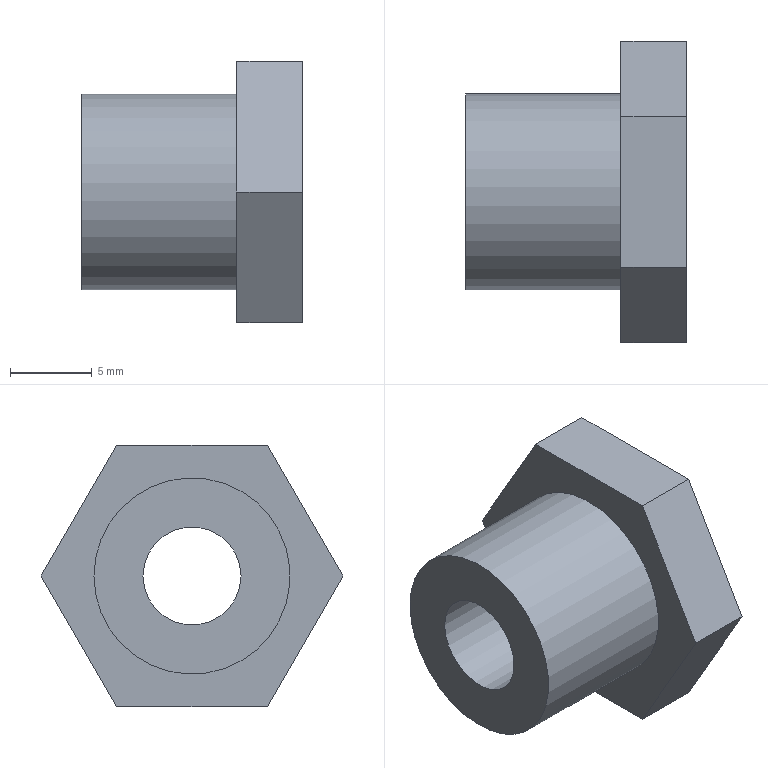Part | STEP file | 1-08.3 | 1 solid | 11 faces | box 13.5 x 18.475 x 16 mm | volume 1580 mm3 | plane 9 | cylinder 2 | commonest cylinder face diameters 6 x1 12 x1
STEP:
#1=CARTESIAN_POINT('',(0.,0.,0.));
#2=DIRECTION('',(0.,0.,1.));
#3=DIRECTION('',(1.,0.,0.));
#4=AXIS2_PLACEMENT_3D('',#1,#2,#3);
#5=CARTESIAN_POINT('',(0.,-4.619,8.));
#6=VERTEX_POINT('',#5);
#7=CARTESIAN_POINT('',(0.,4.619,8.));
#8=VERTEX_POINT('',#7);
#9=CARTESIAN_POINT('',(0.,-4.619,8.));
#10=DIRECTION('',(0.,1.,0.));
#11=VECTOR('',#10,1.);
#12=LINE('',#9,#11);
#13=CARTESIAN_POINT('',(2.,0.,8.));
#14=DIRECTION('',(0.,0.,-1.));
#15=DIRECTION('',(0.,1.,0.));
#16=AXIS2_PLACEMENT_3D('',#13,#14,#15);
#17=PLANE('',#16);
#18=CARTESIAN_POINT('',(-4.619,-2.));
#19=DIRECTION('',(1.,0.));
#20=VECTOR('',#19,1.);
#21=LINE('',#18,#20);
#22=(GEOMETRIC_REPRESENTATION_CONTEXT(2)PARAMETRIC_REPRESENTATION_CONTEXT()REPRESENTATION_CONTEXT('',''));
#23=DEFINITIONAL_REPRESENTATION('',(#21),#22);
#24=PCURVE('',#17,#23);
#25=CARTESIAN_POINT('',(0.,0.,1.238));
#26=DIRECTION('',(-1.,0.,0.));
#27=DIRECTION('',(0.,0.,1.));
#28=AXIS2_PLACEMENT_3D('',#25,#26,#27);
#29=PLANE('',#28);
#30=CARTESIAN_POINT('',(6.762,-4.619));
#31=DIRECTION('',(0.,1.));
#32=VECTOR('',#31,1.);
#33=LINE('',#30,#32);
#34=(GEOMETRIC_REPRESENTATION_CONTEXT(2)PARAMETRIC_REPRESENTATION_CONTEXT()REPRESENTATION_CONTEXT('',''));
#35=DEFINITIONAL_REPRESENTATION('',(#33),#34);
#36=PCURVE('',#29,#35);
#37=SURFACE_CURVE('',#12,(#24,#36),.PCURVE_S1.);
#38=EDGE_CURVE('',#6,#8,#37,.T.);
#39=ORIENTED_EDGE('',*,*,#38,.T.);
#40=CARTESIAN_POINT('',(4.,4.619,8.));
#41=VERTEX_POINT('',#40);
#42=CARTESIAN_POINT('',(0.,4.619,8.));
#43=DIRECTION('',(1.,0.,0.));
#44=VECTOR('',#43,1.);
#45=LINE('',#42,#44);
#46=CARTESIAN_POINT('',(4.619,-2.));
#47=DIRECTION('',(0.,1.));
#48=VECTOR('',#47,1.);
#49=LINE('',#46,#48);
#50=(GEOMETRIC_REPRESENTATION_CONTEXT(2)PARAMETRIC_REPRESENTATION_CONTEXT()REPRESENTATION_CONTEXT('',''));
#51=DEFINITIONAL_REPRESENTATION('',(#49),#50);
#52=PCURVE('',#17,#51);
#53=CARTESIAN_POINT('',(2.,6.928,4.));
#54=DIRECTION('',(0.,-0.866,-0.5));
#55=DIRECTION('',(0.,0.5,-0.866));
#56=AXIS2_PLACEMENT_3D('',#53,#54,#55);
#57=PLANE('',#56);
#58=CARTESIAN_POINT('',(-4.619,-2.));
#59=DIRECTION('',(0.,1.));
#60=VECTOR('',#59,1.);
#61=LINE('',#58,#60);
#62=(GEOMETRIC_REPRESENTATION_CONTEXT(2)PARAMETRIC_REPRESENTATION_CONTEXT()REPRESENTATION_CONTEXT('',''));
#63=DEFINITIONAL_REPRESENTATION('',(#61),#62);
#64=PCURVE('',#57,#63);
#65=SURFACE_CURVE('',#45,(#52,#64),.PCURVE_S1.);
#66=EDGE_CURVE('',#8,#41,#65,.T.);
#67=ORIENTED_EDGE('',*,*,#66,.T.);
#68=CARTESIAN_POINT('',(4.,-4.619,8.));
#69=VERTEX_POINT('',#68);
#70=CARTESIAN_POINT('',(4.,-4.619,8.));
#71=DIRECTION('',(0.,1.,0.));
#72=VECTOR('',#71,1.);
#73=LINE('',#70,#72);
#74=CARTESIAN_POINT('',(-4.619,2.));
#75=DIRECTION('',(1.,0.));
#76=VECTOR('',#75,1.);
#77=LINE('',#74,#76);
#78=(GEOMETRIC_REPRESENTATION_CONTEXT(2)PARAMETRIC_REPRESENTATION_CONTEXT()REPRESENTATION_CONTEXT('',''));
#79=DEFINITIONAL_REPRESENTATION('',(#77),#78);
#80=PCURVE('',#17,#79);
#81=CARTESIAN_POINT('',(4.,0.,1.238));
#82=DIRECTION('',(-1.,0.,0.));
#83=DIRECTION('',(0.,0.,1.));
#84=AXIS2_PLACEMENT_3D('',#81,#82,#83);
#85=PLANE('',#84);
#86=CARTESIAN_POINT('',(6.762,-4.619));
#87=DIRECTION('',(0.,1.));
#88=VECTOR('',#87,1.);
#89=LINE('',#86,#88);
#90=(GEOMETRIC_REPRESENTATION_CONTEXT(2)PARAMETRIC_REPRESENTATION_CONTEXT()REPRESENTATION_CONTEXT('',''));
#91=DEFINITIONAL_REPRESENTATION('',(#89),#90);
#92=PCURVE('',#85,#91);
#93=SURFACE_CURVE('',#73,(#80,#92),.PCURVE_S1.);
#94=EDGE_CURVE('',#69,#41,#93,.T.);
#95=ORIENTED_EDGE('',*,*,#94,.F.);
#96=CARTESIAN_POINT('',(0.,-4.619,8.));
#97=DIRECTION('',(1.,0.,0.));
#98=VECTOR('',#97,1.);
#99=LINE('',#96,#98);
#100=CARTESIAN_POINT('',(-4.619,-2.));
#101=DIRECTION('',(0.,1.));
#102=VECTOR('',#101,1.);
#103=LINE('',#100,#102);
#104=(GEOMETRIC_REPRESENTATION_CONTEXT(2)PARAMETRIC_REPRESENTATION_CONTEXT()REPRESENTATION_CONTEXT('',''));
#105=DEFINITIONAL_REPRESENTATION('',(#103),#104);
#106=PCURVE('',#17,#105);
#107=CARTESIAN_POINT('',(2.,-6.928,4.));
#108=DIRECTION('',(0.,0.866,-0.5));
#109=DIRECTION('',(0.,0.5,0.866));
#110=AXIS2_PLACEMENT_3D('',#107,#108,#109);
#111=PLANE('',#110);
#112=CARTESIAN_POINT('',(4.619,-2.));
#113=DIRECTION('',(0.,1.));
#114=VECTOR('',#113,1.);
#115=LINE('',#112,#114);
#116=(GEOMETRIC_REPRESENTATION_CONTEXT(2)PARAMETRIC_REPRESENTATION_CONTEXT()REPRESENTATION_CONTEXT('',''));
#117=DEFINITIONAL_REPRESENTATION('',(#115),#116);
#118=PCURVE('',#111,#117);
#119=SURFACE_CURVE('',#99,(#106,#118),.PCURVE_S1.);
#120=EDGE_CURVE('',#6,#69,#119,.T.);
#121=ORIENTED_EDGE('',*,*,#120,.F.);
#122=EDGE_LOOP('',(#39,#67,#95,#121));
#123=FACE_BOUND('',#122,.F.);
#124=ADVANCED_FACE('',(#123),#17,.F.);
#125=CARTESIAN_POINT('',(0.,9.238,0.));
#126=VERTEX_POINT('',#125);
#127=CARTESIAN_POINT('',(0.,4.619,8.));
#128=DIRECTION('',(0.,0.5,-0.866));
#129=VECTOR('',#128,1.);
#130=LINE('',#127,#129);
#131=CARTESIAN_POINT('',(-4.619,-2.));
#132=DIRECTION('',(1.,0.));
#133=VECTOR('',#132,1.);
#134=LINE('',#131,#133);
#135=(GEOMETRIC_REPRESENTATION_CONTEXT(2)PARAMETRIC_REPRESENTATION_CONTEXT()REPRESENTATION_CONTEXT('',''));
#136=DEFINITIONAL_REPRESENTATION('',(#134),#135);
#137=PCURVE('',#57,#136);
#138=CARTESIAN_POINT('',(6.762,4.619));
#139=DIRECTION('',(-0.866,0.5));
#140=VECTOR('',#139,1.);
#141=LINE('',#138,#140);
#142=(GEOMETRIC_REPRESENTATION_CONTEXT(2)PARAMETRIC_REPRESENTATION_CONTEXT()REPRESENTATION_CONTEXT('',''));
#143=DEFINITIONAL_REPRESENTATION('',(#141),#142);
#144=PCURVE('',#29,#143);
#145=SURFACE_CURVE('',#130,(#137,#144),.PCURVE_S1.);
#146=EDGE_CURVE('',#8,#126,#145,.T.);
#147=ORIENTED_EDGE('',*,*,#146,.T.);
#148=CARTESIAN_POINT('',(4.,9.238,0.));
#149=VERTEX_POINT('',#148);
#150=CARTESIAN_POINT('',(0.,9.238,0.));
#151=DIRECTION('',(1.,0.,0.));
#152=VECTOR('',#151,1.);
#153=LINE('',#150,#152);
#154=CARTESIAN_POINT('',(4.619,-2.));
#155=DIRECTION('',(0.,1.));
#156=VECTOR('',#155,1.);
#157=LINE('',#154,#156);
#158=(GEOMETRIC_REPRESENTATION_CONTEXT(2)PARAMETRIC_REPRESENTATION_CONTEXT()REPRESENTATION_CONTEXT('',''));
#159=DEFINITIONAL_REPRESENTATION('',(#157),#158);
#160=PCURVE('',#57,#159);
#161=CARTESIAN_POINT('',(2.,6.928,-4.));
#162=DIRECTION('',(0.,-0.866,0.5));
#163=DIRECTION('',(0.,-0.5,-0.866));
#164=AXIS2_PLACEMENT_3D('',#161,#162,#163);
#165=PLANE('',#164);
#166=CARTESIAN_POINT('',(-4.619,-2.));
#167=DIRECTION('',(0.,1.));
#168=VECTOR('',#167,1.);
#169=LINE('',#166,#168);
#170=(GEOMETRIC_REPRESENTATION_CONTEXT(2)PARAMETRIC_REPRESENTATION_CONTEXT()REPRESENTATION_CONTEXT('',''));
#171=DEFINITIONAL_REPRESENTATION('',(#169),#170);
#172=PCURVE('',#165,#171);
#173=SURFACE_CURVE('',#153,(#160,#172),.PCURVE_S1.);
#174=EDGE_CURVE('',#126,#149,#173,.T.);
#175=ORIENTED_EDGE('',*,*,#174,.T.);
#176=CARTESIAN_POINT('',(4.,4.619,8.));
#177=DIRECTION('',(0.,0.5,-0.866));
#178=VECTOR('',#177,1.);
#179=LINE('',#176,#178);
#180=CARTESIAN_POINT('',(-4.619,2.));
#181=DIRECTION('',(1.,0.));
#182=VECTOR('',#181,1.);
#183=LINE('',#180,#182);
#184=(GEOMETRIC_REPRESENTATION_CONTEXT(2)PARAMETRIC_REPRESENTATION_CONTEXT()REPRESENTATION_CONTEXT('',''));
#185=DEFINITIONAL_REPRESENTATION('',(#183),#184);
#186=PCURVE('',#57,#185);
#187=CARTESIAN_POINT('',(6.762,4.619));
#188=DIRECTION('',(-0.866,0.5));
#189=VECTOR('',#188,1.);
#190=LINE('',#187,#189);
#191=(GEOMETRIC_REPRESENTATION_CONTEXT(2)PARAMETRIC_REPRESENTATION_CONTEXT()REPRESENTATION_CONTEXT('',''));
#192=DEFINITIONAL_REPRESENTATION('',(#190),#191);
#193=PCURVE('',#85,#192);
#194=SURFACE_CURVE('',#179,(#186,#193),.PCURVE_S1.);
#195=EDGE_CURVE('',#41,#149,#194,.T.);
#196=ORIENTED_EDGE('',*,*,#195,.F.);
#197=ORIENTED_EDGE('',*,*,#66,.F.);
#198=EDGE_LOOP('',(#147,#175,#196,#197));
#199=FACE_BOUND('',#198,.F.);
#200=ADVANCED_FACE('',(#199),#57,.F.);
#201=CARTESIAN_POINT('',(0.,4.619,-8.));
#202=VERTEX_POINT('',#201);
#203=CARTESIAN_POINT('',(0.,9.238,0.));
#204=DIRECTION('',(0.,-0.5,-0.866));
#205=VECTOR('',#204,1.);
#206=LINE('',#203,#205);
#207=CARTESIAN_POINT('',(-4.619,-2.));
#208=DIRECTION('',(1.,0.));
#209=VECTOR('',#208,1.);
#210=LINE('',#207,#209);
#211=(GEOMETRIC_REPRESENTATION_CONTEXT(2)PARAMETRIC_REPRESENTATION_CONTEXT()REPRESENTATION_CONTEXT('',''));
#212=DEFINITIONAL_REPRESENTATION('',(#210),#211);
#213=PCURVE('',#165,#212);
#214=CARTESIAN_POINT('',(-1.238,9.238));
#215=DIRECTION('',(-0.866,-0.5));
#216=VECTOR('',#215,1.);
#217=LINE('',#214,#216);
#218=(GEOMETRIC_REPRESENTATION_CONTEXT(2)PARAMETRIC_REPRESENTATION_CONTEXT()REPRESENTATION_CONTEXT('',''));
#219=DEFINITIONAL_REPRESENTATION('',(#217),#218);
#220=PCURVE('',#29,#219);
#221=SURFACE_CURVE('',#206,(#213,#220),.PCURVE_S1.);
#222=EDGE_CURVE('',#126,#202,#221,.T.);
#223=ORIENTED_EDGE('',*,*,#222,.T.);
#224=CARTESIAN_POINT('',(4.,4.619,-8.));
#225=VERTEX_POINT('',#224);
#226=CARTESIAN_POINT('',(0.,4.619,-8.));
#227=DIRECTION('',(1.,0.,0.));
#228=VECTOR('',#227,1.);
#229=LINE('',#226,#228);
#230=CARTESIAN_POINT('',(4.619,-2.));
#231=DIRECTION('',(0.,1.));
#232=VECTOR('',#231,1.);
#233=LINE('',#230,#232);
#234=(GEOMETRIC_REPRESENTATION_CONTEXT(2)PARAMETRIC_REPRESENTATION_CONTEXT()REPRESENTATION_CONTEXT('',''));
#235=DEFINITIONAL_REPRESENTATION('',(#233),#234);
#236=PCURVE('',#165,#235);
#237=CARTESIAN_POINT('',(2.,0.,-8.));
#238=DIRECTION('',(0.,0.,1.));
#239=DIRECTION('',(0.,-1.,0.));
#240=AXIS2_PLACEMENT_3D('',#237,#238,#239);
#241=PLANE('',#240);
#242=CARTESIAN_POINT('',(-4.619,-2.));
#243=DIRECTION('',(0.,1.));
#244=VECTOR('',#243,1.);
#245=LINE('',#242,#244);
#246=(GEOMETRIC_REPRESENTATION_CONTEXT(2)PARAMETRIC_REPRESENTATION_CONTEXT()REPRESENTATION_CONTEXT('',''));
#247=DEFINITIONAL_REPRESENTATION('',(#245),#246);
#248=PCURVE('',#241,#247);
#249=SURFACE_CURVE('',#229,(#236,#248),.PCURVE_S1.);
#250=EDGE_CURVE('',#202,#225,#249,.T.);
#251=ORIENTED_EDGE('',*,*,#250,.T.);
#252=CARTESIAN_POINT('',(4.,9.238,0.));
#253=DIRECTION('',(0.,-0.5,-0.866));
#254=VECTOR('',#253,1.);
#255=LINE('',#252,#254);
#256=CARTESIAN_POINT('',(-4.619,2.));
#257=DIRECTION('',(1.,0.));
#258=VECTOR('',#257,1.);
#259=LINE('',#256,#258);
#260=(GEOMETRIC_REPRESENTATION_CONTEXT(2)PARAMETRIC_REPRESENTATION_CONTEXT()REPRESENTATION_CONTEXT('',''));
#261=DEFINITIONAL_REPRESENTATION('',(#259),#260);
#262=PCURVE('',#165,#261);
#263=CARTESIAN_POINT('',(-1.238,9.238));
#264=DIRECTION('',(-0.866,-0.5));
#265=VECTOR('',#264,1.);
#266=LINE('',#263,#265);
#267=(GEOMETRIC_REPRESENTATION_CONTEXT(2)PARAMETRIC_REPRESENTATION_CONTEXT()REPRESENTATION_CONTEXT('',''));
#268=DEFINITIONAL_REPRESENTATION('',(#266),#267);
#269=PCURVE('',#85,#268);
#270=SURFACE_CURVE('',#255,(#262,#269),.PCURVE_S1.);
#271=EDGE_CURVE('',#149,#225,#270,.T.);
#272=ORIENTED_EDGE('',*,*,#271,.F.);
#273=ORIENTED_EDGE('',*,*,#174,.F.);
#274=EDGE_LOOP('',(#223,#251,#272,#273));
#275=FACE_BOUND('',#274,.F.);
#276=ADVANCED_FACE('',(#275),#165,.F.);
#277=CARTESIAN_POINT('',(0.,-4.619,-8.));
#278=VERTEX_POINT('',#277);
#279=CARTESIAN_POINT('',(0.,4.619,-8.));
#280=DIRECTION('',(0.,-1.,0.));
#281=VECTOR('',#280,1.);
#282=LINE('',#279,#281);
#283=CARTESIAN_POINT('',(-4.619,-2.));
#284=DIRECTION('',(1.,0.));
#285=VECTOR('',#284,1.);
#286=LINE('',#283,#285);
#287=(GEOMETRIC_REPRESENTATION_CONTEXT(2)PARAMETRIC_REPRESENTATION_CONTEXT()REPRESENTATION_CONTEXT('',''));
#288=DEFINITIONAL_REPRESENTATION('',(#286),#287);
#289=PCURVE('',#241,#288);
#290=CARTESIAN_POINT('',(-9.238,4.619));
#291=DIRECTION('',(0.,-1.));
#292=VECTOR('',#291,1.);
#293=LINE('',#290,#292);
#294=(GEOMETRIC_REPRESENTATION_CONTEXT(2)PARAMETRIC_REPRESENTATION_CONTEXT()REPRESENTATION_CONTEXT('',''));
#295=DEFINITIONAL_REPRESENTATION('',(#293),#294);
#296=PCURVE('',#29,#295);
#297=SURFACE_CURVE('',#282,(#289,#296),.PCURVE_S1.);
#298=EDGE_CURVE('',#202,#278,#297,.T.);
#299=ORIENTED_EDGE('',*,*,#298,.T.);
#300=CARTESIAN_POINT('',(4.,-4.619,-8.));
#301=VERTEX_POINT('',#300);
#302=CARTESIAN_POINT('',(0.,-4.619,-8.));
#303=DIRECTION('',(1.,0.,0.));
#304=VECTOR('',#303,1.);
#305=LINE('',#302,#304);
#306=CARTESIAN_POINT('',(4.619,-2.));
#307=DIRECTION('',(0.,1.));
#308=VECTOR('',#307,1.);
#309=LINE('',#306,#308);
#310=(GEOMETRIC_REPRESENTATION_CONTEXT(2)PARAMETRIC_REPRESENTATION_CONTEXT()REPRESENTATION_CONTEXT('',''));
#311=DEFINITIONAL_REPRESENTATION('',(#309),#310);
#312=PCURVE('',#241,#311);
#313=CARTESIAN_POINT('',(2.,-6.928,-4.));
#314=DIRECTION('',(0.,0.866,0.5));
#315=DIRECTION('',(0.,-0.5,0.866));
#316=AXIS2_PLACEMENT_3D('',#313,#314,#315);
#317=PLANE('',#316);
#318=CARTESIAN_POINT('',(-4.619,-2.));
#319=DIRECTION('',(0.,1.));
#320=VECTOR('',#319,1.);
#321=LINE('',#318,#320);
#322=(GEOMETRIC_REPRESENTATION_CONTEXT(2)PARAMETRIC_REPRESENTATION_CONTEXT()REPRESENTATION_CONTEXT('',''));
#323=DEFINITIONAL_REPRESENTATION('',(#321),#322);
#324=PCURVE('',#317,#323);
#325=SURFACE_CURVE('',#305,(#312,#324),.PCURVE_S1.);
#326=EDGE_CURVE('',#278,#301,#325,.T.);
#327=ORIENTED_EDGE('',*,*,#326,.T.);
#328=CARTESIAN_POINT('',(4.,4.619,-8.));
#329=DIRECTION('',(0.,-1.,0.));
#330=VECTOR('',#329,1.);
#331=LINE('',#328,#330);
#332=CARTESIAN_POINT('',(-4.619,2.));
#333=DIRECTION('',(1.,0.));
#334=VECTOR('',#333,1.);
#335=LINE('',#332,#334);
#336=(GEOMETRIC_REPRESENTATION_CONTEXT(2)PARAMETRIC_REPRESENTATION_CONTEXT()REPRESENTATION_CONTEXT('',''));
#337=DEFINITIONAL_REPRESENTATION('',(#335),#336);
#338=PCURVE('',#241,#337);
#339=CARTESIAN_POINT('',(-9.238,4.619));
#340=DIRECTION('',(0.,-1.));
#341=VECTOR('',#340,1.);
#342=LINE('',#339,#341);
#343=(GEOMETRIC_REPRESENTATION_CONTEXT(2)PARAMETRIC_REPRESENTATION_CONTEXT()REPRESENTATION_CONTEXT('',''));
#344=DEFINITIONAL_REPRESENTATION('',(#342),#343);
#345=PCURVE('',#85,#344);
#346=SURFACE_CURVE('',#331,(#338,#345),.PCURVE_S1.);
#347=EDGE_CURVE('',#225,#301,#346,.T.);
#348=ORIENTED_EDGE('',*,*,#347,.F.);
#349=ORIENTED_EDGE('',*,*,#250,.F.);
#350=EDGE_LOOP('',(#299,#327,#348,#349));
#351=FACE_BOUND('',#350,.F.);
#352=ADVANCED_FACE('',(#351),#241,.F.);
#353=CARTESIAN_POINT('',(0.,-9.238,0.));
#354=VERTEX_POINT('',#353);
#355=CARTESIAN_POINT('',(0.,-4.619,-8.));
#356=DIRECTION('',(0.,-0.5,0.866));
#357=VECTOR('',#356,1.);
#358=LINE('',#355,#357);
#359=CARTESIAN_POINT('',(-4.619,-2.));
#360=DIRECTION('',(1.,0.));
#361=VECTOR('',#360,1.);
#362=LINE('',#359,#361);
#363=(GEOMETRIC_REPRESENTATION_CONTEXT(2)PARAMETRIC_REPRESENTATION_CONTEXT()REPRESENTATION_CONTEXT('',''));
#364=DEFINITIONAL_REPRESENTATION('',(#362),#363);
#365=PCURVE('',#317,#364);
#366=CARTESIAN_POINT('',(-9.238,-4.619));
#367=DIRECTION('',(0.866,-0.5));
#368=VECTOR('',#367,1.);
#369=LINE('',#366,#368);
#370=(GEOMETRIC_REPRESENTATION_CONTEXT(2)PARAMETRIC_REPRESENTATION_CONTEXT()REPRESENTATION_CONTEXT('',''));
#371=DEFINITIONAL_REPRESENTATION('',(#369),#370);
#372=PCURVE('',#29,#371);
#373=SURFACE_CURVE('',#358,(#365,#372),.PCURVE_S1.);
#374=EDGE_CURVE('',#278,#354,#373,.T.);
#375=ORIENTED_EDGE('',*,*,#374,.T.);
#376=CARTESIAN_POINT('',(4.,-9.238,0.));
#377=VERTEX_POINT('',#376);
#378=CARTESIAN_POINT('',(0.,-9.238,0.));
#379=DIRECTION('',(1.,0.,0.));
#380=VECTOR('',#379,1.);
#381=LINE('',#378,#380);
#382=CARTESIAN_POINT('',(4.619,-2.));
#383=DIRECTION('',(0.,1.));
#384=VECTOR('',#383,1.);
#385=LINE('',#382,#384);
#386=(GEOMETRIC_REPRESENTATION_CONTEXT(2)PARAMETRIC_REPRESENTATION_CONTEXT()REPRESENTATION_CONTEXT('',''));
#387=DEFINITIONAL_REPRESENTATION('',(#385),#386);
#388=PCURVE('',#317,#387);
#389=CARTESIAN_POINT('',(-4.619,-2.));
#390=DIRECTION('',(0.,1.));
#391=VECTOR('',#390,1.);
#392=LINE('',#389,#391);
#393=(GEOMETRIC_REPRESENTATION_CONTEXT(2)PARAMETRIC_REPRESENTATION_CONTEXT()REPRESENTATION_CONTEXT('',''));
#394=DEFINITIONAL_REPRESENTATION('',(#392),#393);
#395=PCURVE('',#111,#394);
#396=SURFACE_CURVE('',#381,(#388,#395),.PCURVE_S1.);
#397=EDGE_CURVE('',#354,#377,#396,.T.);
#398=ORIENTED_EDGE('',*,*,#397,.T.);
#399=CARTESIAN_POINT('',(4.,-4.619,-8.));
#400=DIRECTION('',(0.,-0.5,0.866));
#401=VECTOR('',#400,1.);
#402=LINE('',#399,#401);
#403=CARTESIAN_POINT('',(-4.619,2.));
#404=DIRECTION('',(1.,0.));
#405=VECTOR('',#404,1.);
#406=LINE('',#403,#405);
#407=(GEOMETRIC_REPRESENTATION_CONTEXT(2)PARAMETRIC_REPRESENTATION_CONTEXT()REPRESENTATION_CONTEXT('',''));
#408=DEFINITIONAL_REPRESENTATION('',(#406),#407);
#409=PCURVE('',#317,#408);
#410=CARTESIAN_POINT('',(-9.238,-4.619));
#411=DIRECTION('',(0.866,-0.5));
#412=VECTOR('',#411,1.);
#413=LINE('',#410,#412);
#414=(GEOMETRIC_REPRESENTATION_CONTEXT(2)PARAMETRIC_REPRESENTATION_CONTEXT()REPRESENTATION_CONTEXT('',''));
#415=DEFINITIONAL_REPRESENTATION('',(#413),#414);
#416=PCURVE('',#85,#415);
#417=SURFACE_CURVE('',#402,(#409,#416),.PCURVE_S1.);
#418=EDGE_CURVE('',#301,#377,#417,.T.);
#419=ORIENTED_EDGE('',*,*,#418,.F.);
#420=ORIENTED_EDGE('',*,*,#326,.F.);
#421=EDGE_LOOP('',(#375,#398,#419,#420));
#422=FACE_BOUND('',#421,.F.);
#423=ADVANCED_FACE('',(#422),#317,.F.);
#424=CARTESIAN_POINT('',(0.,-9.238,0.));
#425=DIRECTION('',(0.,0.5,0.866));
#426=VECTOR('',#425,1.);
#427=LINE('',#424,#426);
#428=CARTESIAN_POINT('',(-4.619,-2.));
#429=DIRECTION('',(1.,0.));
#430=VECTOR('',#429,1.);
#431=LINE('',#428,#430);
#432=(GEOMETRIC_REPRESENTATION_CONTEXT(2)PARAMETRIC_REPRESENTATION_CONTEXT()REPRESENTATION_CONTEXT('',''));
#433=DEFINITIONAL_REPRESENTATION('',(#431),#432);
#434=PCURVE('',#111,#433);
#435=CARTESIAN_POINT('',(-1.238,-9.238));
#436=DIRECTION('',(0.866,0.5));
#437=VECTOR('',#436,1.);
#438=LINE('',#435,#437);
#439=(GEOMETRIC_REPRESENTATION_CONTEXT(2)PARAMETRIC_REPRESENTATION_CONTEXT()REPRESENTATION_CONTEXT('',''));
#440=DEFINITIONAL_REPRESENTATION('',(#438),#439);
#441=PCURVE('',#29,#440);
#442=SURFACE_CURVE('',#427,(#434,#441),.PCURVE_S1.);
#443=EDGE_CURVE('',#354,#6,#442,.T.);
#444=ORIENTED_EDGE('',*,*,#443,.T.);
#445=ORIENTED_EDGE('',*,*,#120,.T.);
#446=CARTESIAN_POINT('',(4.,-9.238,0.));
#447=DIRECTION('',(0.,0.5,0.866));
#448=VECTOR('',#447,1.);
#449=LINE('',#446,#448);
#450=CARTESIAN_POINT('',(-4.619,2.));
#451=DIRECTION('',(1.,0.));
#452=VECTOR('',#451,1.);
#453=LINE('',#450,#452);
#454=(GEOMETRIC_REPRESENTATION_CONTEXT(2)PARAMETRIC_REPRESENTATION_CONTEXT()REPRESENTATION_CONTEXT('',''));
#455=DEFINITIONAL_REPRESENTATION('',(#453),#454);
#456=PCURVE('',#111,#455);
#457=CARTESIAN_POINT('',(-1.238,-9.238));
#458=DIRECTION('',(0.866,0.5));
#459=VECTOR('',#458,1.);
#460=LINE('',#457,#459);
#461=(GEOMETRIC_REPRESENTATION_CONTEXT(2)PARAMETRIC_REPRESENTATION_CONTEXT()REPRESENTATION_CONTEXT('',''));
#462=DEFINITIONAL_REPRESENTATION('',(#460),#461);
#463=PCURVE('',#85,#462);
#464=SURFACE_CURVE('',#449,(#456,#463),.PCURVE_S1.);
#465=EDGE_CURVE('',#377,#69,#464,.T.);
#466=ORIENTED_EDGE('',*,*,#465,.F.);
#467=ORIENTED_EDGE('',*,*,#397,.F.);
#468=EDGE_LOOP('',(#444,#445,#466,#467));
#469=FACE_BOUND('',#468,.F.);
#470=ADVANCED_FACE('',(#469),#111,.F.);
#471=ORIENTED_EDGE('',*,*,#38,.T.);
#472=ORIENTED_EDGE('',*,*,#146,.T.);
#473=ORIENTED_EDGE('',*,*,#222,.T.);
#474=ORIENTED_EDGE('',*,*,#298,.T.);
#475=ORIENTED_EDGE('',*,*,#374,.T.);
#476=ORIENTED_EDGE('',*,*,#443,.T.);
#477=EDGE_LOOP('',(#471,#472,#473,#474,#475,#476));
#478=FACE_BOUND('',#477,.T.);
#479=CARTESIAN_POINT('',(0.,6.,0.));
#480=VERTEX_POINT('',#479);
#481=CARTESIAN_POINT('',(0.,0.,0.));
#482=DIRECTION('',(1.,0.,0.));
#483=DIRECTION('',(0.,1.,0.));
#484=AXIS2_PLACEMENT_3D('',#481,#482,#483);
#485=CIRCLE('',#484,6.);
#486=CARTESIAN_POINT('',(-1.238,6.));
#487=CARTESIAN_POINT('',(9.155,6.));
#488=CARTESIAN_POINT('',(3.959,-3.));
#489=CARTESIAN_POINT('',(-1.238,-12.));
#490=CARTESIAN_POINT('',(-6.434,-3.));
#491=CARTESIAN_POINT('',(-11.63,6.));
#492=CARTESIAN_POINT('',(-1.238,6.));
#493=(BOUNDED_CURVE()B_SPLINE_CURVE(2,(#486,#487,#488,#489,#490,#491,#492),.UNSPECIFIED.,.T.,.F.)B_SPLINE_CURVE_WITH_KNOTS((1,2,2,2,2,1),(-2.094,0.,2.094,4.189,6.283,8.378),.UNSPECIFIED.)CURVE()GEOMETRIC_REPRESENTATION_ITEM()RATIONAL_B_SPLINE_CURVE((1.,0.5,1.,0.5,1.,0.5,1.))REPRESENTATION_ITEM(''));
#494=(GEOMETRIC_REPRESENTATION_CONTEXT(2)PARAMETRIC_REPRESENTATION_CONTEXT()REPRESENTATION_CONTEXT('',''));
#495=DEFINITIONAL_REPRESENTATION('',(#493),#494);
#496=PCURVE('',#29,#495);
#497=CARTESIAN_POINT('',(0.,0.,0.));
#498=DIRECTION('',(-1.,0.,0.));
#499=DIRECTION('',(0.,1.,0.));
#500=AXIS2_PLACEMENT_3D('',#497,#498,#499);
#501=CYLINDRICAL_SURFACE('',#500,6.);
#502=CARTESIAN_POINT('',(6.283,0.));
#503=DIRECTION('',(-1.,0.));
#504=VECTOR('',#503,1.);
#505=LINE('',#502,#504);
#506=(GEOMETRIC_REPRESENTATION_CONTEXT(2)PARAMETRIC_REPRESENTATION_CONTEXT()REPRESENTATION_CONTEXT('',''));
#507=DEFINITIONAL_REPRESENTATION('',(#505),#506);
#508=PCURVE('',#501,#507);
#509=SURFACE_CURVE('',#485,(#496,#508),.PCURVE_S1.);
#510=EDGE_CURVE('',#480,#480,#509,.T.);
#511=ORIENTED_EDGE('',*,*,#510,.T.);
#512=EDGE_LOOP('',(#511));
#513=FACE_BOUND('',#512,.T.);
#514=ADVANCED_FACE('',(#478,#513),#29,.T.);
#515=CARTESIAN_POINT('',(-9.5,6.,0.));
#516=VERTEX_POINT('',#515);
#517=CARTESIAN_POINT('',(0.,6.,0.));
#518=DIRECTION('',(-1.,0.,0.));
#519=VECTOR('',#518,1.);
#520=LINE('',#517,#519);
#521=CARTESIAN_POINT('',(6.283,0.));
#522=DIRECTION('',(0.,1.));
#523=VECTOR('',#522,1.);
#524=LINE('',#521,#523);
#525=(GEOMETRIC_REPRESENTATION_CONTEXT(2)PARAMETRIC_REPRESENTATION_CONTEXT()REPRESENTATION_CONTEXT('',''));
#526=DEFINITIONAL_REPRESENTATION('',(#524),#525);
#527=PCURVE('',#501,#526);
#528=CARTESIAN_POINT('',(0.,0.));
#529=DIRECTION('',(0.,1.));
#530=VECTOR('',#529,1.);
#531=LINE('',#528,#530);
#532=(GEOMETRIC_REPRESENTATION_CONTEXT(2)PARAMETRIC_REPRESENTATION_CONTEXT()REPRESENTATION_CONTEXT('',''));
#533=DEFINITIONAL_REPRESENTATION('',(#531),#532);
#534=PCURVE('',#501,#533);
#535=SEAM_CURVE('',#520,(#527,#534),.PCURVE_S1.);
#536=EDGE_CURVE('',#480,#516,#535,.T.);
#537=ORIENTED_EDGE('',*,*,#536,.T.);
#538=CARTESIAN_POINT('',(-9.5,0.,0.));
#539=DIRECTION('',(1.,0.,0.));
#540=DIRECTION('',(0.,1.,0.));
#541=AXIS2_PLACEMENT_3D('',#538,#539,#540);
#542=CIRCLE('',#541,6.);
#543=CARTESIAN_POINT('',(6.283,9.5));
#544=DIRECTION('',(-1.,0.));
#545=VECTOR('',#544,1.);
#546=LINE('',#543,#545);
#547=(GEOMETRIC_REPRESENTATION_CONTEXT(2)PARAMETRIC_REPRESENTATION_CONTEXT()REPRESENTATION_CONTEXT('',''));
#548=DEFINITIONAL_REPRESENTATION('',(#546),#547);
#549=PCURVE('',#501,#548);
#550=CARTESIAN_POINT('',(-9.5,-1.608,0.));
#551=DIRECTION('',(1.,0.,0.));
#552=DIRECTION('',(0.,0.,-1.));
#553=AXIS2_PLACEMENT_3D('',#550,#551,#552);
#554=PLANE('',#553);
#555=CARTESIAN_POINT('',(0.,1.608));
#556=DIRECTION('',(0.,1.));
#557=AXIS2_PLACEMENT_2D('',#555,#556);
#558=CIRCLE('',#557,6.);
#559=(GEOMETRIC_REPRESENTATION_CONTEXT(2)PARAMETRIC_REPRESENTATION_CONTEXT()REPRESENTATION_CONTEXT('',''));
#560=DEFINITIONAL_REPRESENTATION('',(#558),#559);
#561=PCURVE('',#554,#560);
#562=SURFACE_CURVE('',#542,(#549,#561),.PCURVE_S1.);
#563=EDGE_CURVE('',#516,#516,#562,.T.);
#564=ORIENTED_EDGE('',*,*,#563,.T.);
#565=ORIENTED_EDGE('',*,*,#536,.F.);
#566=ORIENTED_EDGE('',*,*,#510,.F.);
#567=EDGE_LOOP('',(#537,#564,#565,#566));
#568=FACE_BOUND('',#567,.T.);
#569=ADVANCED_FACE('',(#568),#501,.T.);
#570=ORIENTED_EDGE('',*,*,#94,.T.);
#571=ORIENTED_EDGE('',*,*,#195,.T.);
#572=ORIENTED_EDGE('',*,*,#271,.T.);
#573=ORIENTED_EDGE('',*,*,#347,.T.);
#574=ORIENTED_EDGE('',*,*,#418,.T.);
#575=ORIENTED_EDGE('',*,*,#465,.T.);
#576=EDGE_LOOP('',(#570,#571,#572,#573,#574,#575));
#577=FACE_BOUND('',#576,.F.);
#578=CARTESIAN_POINT('',(4.,3.,0.));
#579=VERTEX_POINT('',#578);
#580=CARTESIAN_POINT('',(4.,0.,0.));
#581=DIRECTION('',(1.,0.,0.));
#582=DIRECTION('',(0.,1.,0.));
#583=AXIS2_PLACEMENT_3D('',#580,#581,#582);
#584=CIRCLE('',#583,3.);
#585=CARTESIAN_POINT('',(-1.238,3.));
#586=CARTESIAN_POINT('',(3.959,3.));
#587=CARTESIAN_POINT('',(1.36,-1.5));
#588=CARTESIAN_POINT('',(-1.238,-6.));
#589=CARTESIAN_POINT('',(-3.836,-1.5));
#590=CARTESIAN_POINT('',(-6.434,3.));
#591=CARTESIAN_POINT('',(-1.238,3.));
#592=(BOUNDED_CURVE()B_SPLINE_CURVE(2,(#585,#586,#587,#588,#589,#590,#591),.UNSPECIFIED.,.T.,.F.)B_SPLINE_CURVE_WITH_KNOTS((1,2,2,2,2,1),(-2.094,0.,2.094,4.189,6.283,8.378),.UNSPECIFIED.)CURVE()GEOMETRIC_REPRESENTATION_ITEM()RATIONAL_B_SPLINE_CURVE((1.,0.5,1.,0.5,1.,0.5,1.))REPRESENTATION_ITEM(''));
#593=(GEOMETRIC_REPRESENTATION_CONTEXT(2)PARAMETRIC_REPRESENTATION_CONTEXT()REPRESENTATION_CONTEXT('',''));
#594=DEFINITIONAL_REPRESENTATION('',(#592),#593);
#595=PCURVE('',#85,#594);
#596=CARTESIAN_POINT('',(4.,0.,0.));
#597=DIRECTION('',(-1.,0.,0.));
#598=DIRECTION('',(0.,1.,0.));
#599=AXIS2_PLACEMENT_3D('',#596,#597,#598);
#600=CYLINDRICAL_SURFACE('',#599,3.);
#601=CARTESIAN_POINT('',(6.283,0.));
#602=DIRECTION('',(-1.,0.));
#603=VECTOR('',#602,1.);
#604=LINE('',#601,#603);
#605=(GEOMETRIC_REPRESENTATION_CONTEXT(2)PARAMETRIC_REPRESENTATION_CONTEXT()REPRESENTATION_CONTEXT('',''));
#606=DEFINITIONAL_REPRESENTATION('',(#604),#605);
#607=PCURVE('',#600,#606);
#608=SURFACE_CURVE('',#584,(#595,#607),.PCURVE_S1.);
#609=EDGE_CURVE('',#579,#579,#608,.T.);
#610=ORIENTED_EDGE('',*,*,#609,.T.);
#611=EDGE_LOOP('',(#610));
#612=FACE_BOUND('',#611,.F.);
#613=ADVANCED_FACE('',(#577,#612),#85,.F.);
#614=ORIENTED_EDGE('',*,*,#563,.T.);
#615=EDGE_LOOP('',(#614));
#616=FACE_BOUND('',#615,.F.);
#617=CARTESIAN_POINT('',(-9.5,3.,0.));
#618=VERTEX_POINT('',#617);
#619=CARTESIAN_POINT('',(-9.5,0.,0.));
#620=DIRECTION('',(1.,0.,0.));
#621=DIRECTION('',(0.,1.,0.));
#622=AXIS2_PLACEMENT_3D('',#619,#620,#621);
#623=CIRCLE('',#622,3.);
#624=CARTESIAN_POINT('',(0.,1.608));
#625=DIRECTION('',(0.,1.));
#626=AXIS2_PLACEMENT_2D('',#624,#625);
#627=CIRCLE('',#626,3.);
#628=(GEOMETRIC_REPRESENTATION_CONTEXT(2)PARAMETRIC_REPRESENTATION_CONTEXT()REPRESENTATION_CONTEXT('',''));
#629=DEFINITIONAL_REPRESENTATION('',(#627),#628);
#630=PCURVE('',#554,#629);
#631=CARTESIAN_POINT('',(6.283,13.5));
#632=DIRECTION('',(-1.,0.));
#633=VECTOR('',#632,1.);
#634=LINE('',#631,#633);
#635=(GEOMETRIC_REPRESENTATION_CONTEXT(2)PARAMETRIC_REPRESENTATION_CONTEXT()REPRESENTATION_CONTEXT('',''));
#636=DEFINITIONAL_REPRESENTATION('',(#634),#635);
#637=PCURVE('',#600,#636);
#638=SURFACE_CURVE('',#623,(#630,#637),.PCURVE_S1.);
#639=EDGE_CURVE('',#618,#618,#638,.T.);
#640=ORIENTED_EDGE('',*,*,#639,.F.);
#641=EDGE_LOOP('',(#640));
#642=FACE_BOUND('',#641,.F.);
#643=ADVANCED_FACE('',(#616,#642),#554,.F.);
#644=CARTESIAN_POINT('',(4.,3.,0.));
#645=DIRECTION('',(-1.,0.,0.));
#646=VECTOR('',#645,1.);
#647=LINE('',#644,#646);
#648=CARTESIAN_POINT('',(6.283,0.));
#649=DIRECTION('',(0.,1.));
#650=VECTOR('',#649,1.);
#651=LINE('',#648,#650);
#652=(GEOMETRIC_REPRESENTATION_CONTEXT(2)PARAMETRIC_REPRESENTATION_CONTEXT()REPRESENTATION_CONTEXT('',''));
#653=DEFINITIONAL_REPRESENTATION('',(#651),#652);
#654=PCURVE('',#600,#653);
#655=CARTESIAN_POINT('',(0.,0.));
#656=DIRECTION('',(0.,1.));
#657=VECTOR('',#656,1.);
#658=LINE('',#655,#657);
#659=(GEOMETRIC_REPRESENTATION_CONTEXT(2)PARAMETRIC_REPRESENTATION_CONTEXT()REPRESENTATION_CONTEXT('',''));
#660=DEFINITIONAL_REPRESENTATION('',(#658),#659);
#661=PCURVE('',#600,#660);
#662=SEAM_CURVE('',#647,(#654,#661),.PCURVE_S1.);
#663=EDGE_CURVE('',#579,#618,#662,.T.);
#664=ORIENTED_EDGE('',*,*,#663,.T.);
#665=ORIENTED_EDGE('',*,*,#639,.T.);
#666=ORIENTED_EDGE('',*,*,#663,.F.);
#667=ORIENTED_EDGE('',*,*,#609,.F.);
#668=EDGE_LOOP('',(#664,#665,#666,#667));
#669=FACE_BOUND('',#668,.F.);
#670=ADVANCED_FACE('',(#669),#600,.F.);
#671=CLOSED_SHELL('',(#124,#200,#276,#352,#423,#470,#514,#569,#613,#643,#670));
#672=MANIFOLD_SOLID_BREP('',#671);
#673=(LENGTH_UNIT()NAMED_UNIT(*)SI_UNIT(.MILLI.,.METRE.));
#674=UNCERTAINTY_MEASURE_WITH_UNIT(LENGTH_MEASURE(0.0000001),#673,'','');
#675=(NAMED_UNIT(*)PLANE_ANGLE_UNIT()SI_UNIT($,.RADIAN.));
#676=(NAMED_UNIT(*)SI_UNIT($,.STERADIAN.)SOLID_ANGLE_UNIT());
#677=(GEOMETRIC_REPRESENTATION_CONTEXT(3)GLOBAL_UNCERTAINTY_ASSIGNED_CONTEXT((#674))GLOBAL_UNIT_ASSIGNED_CONTEXT((#673,#675,#676))REPRESENTATION_CONTEXT('',''));
#678=ADVANCED_BREP_SHAPE_REPRESENTATION('',(#4,#672),#677);